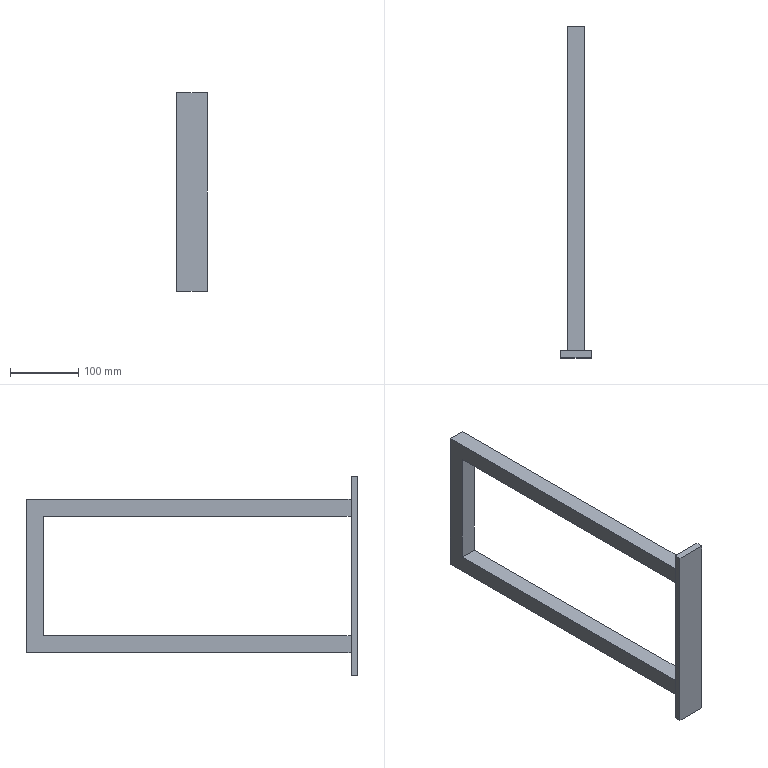Part | SolidWorks | features BaseBody 1 | 1 solid | 14 faces | box 45 x 485 x 290 mm | volume 833625 mm3 | plane 14
STEP:
#1=CARTESIAN_POINT('',(12.5,485.,-112.5));
#2=VERTEX_POINT('',#1);
#3=CARTESIAN_POINT('',(12.5,10.,-112.5));
#4=VERTEX_POINT('',#3);
#5=CARTESIAN_POINT('',(12.5,460.,-112.5));
#6=DIRECTION('',(0.,-1.,0.));
#7=VECTOR('',#6,1000.);
#8=LINE('',#5,#7);
#9=EDGE_CURVE('',#2,#4,#8,.T.);
#10=ORIENTED_EDGE('',*,*,#9,.F.);
#11=CARTESIAN_POINT('',(12.5,485.,112.5));
#12=VERTEX_POINT('',#11);
#13=CARTESIAN_POINT('',(12.5,485.,-112.5));
#14=DIRECTION('',(0.,0.,-1.));
#15=VECTOR('',#14,1000.);
#16=LINE('',#13,#15);
#17=EDGE_CURVE('',#12,#2,#16,.T.);
#18=ORIENTED_EDGE('',*,*,#17,.F.);
#19=CARTESIAN_POINT('',(12.5,10.,112.5));
#20=VERTEX_POINT('',#19);
#21=CARTESIAN_POINT('',(12.5,460.,112.5));
#22=DIRECTION('',(0.,1.,0.));
#23=VECTOR('',#22,1000.);
#24=LINE('',#21,#23);
#25=EDGE_CURVE('',#20,#12,#24,.T.);
#26=ORIENTED_EDGE('',*,*,#25,.F.);
#27=CARTESIAN_POINT('',(12.5,10.,87.5));
#28=VERTEX_POINT('',#27);
#29=CARTESIAN_POINT('',(12.5,10.,-112.5));
#30=DIRECTION('',(0.,0.,1.));
#31=VECTOR('',#30,1000.);
#32=LINE('',#29,#31);
#33=EDGE_CURVE('',#28,#20,#32,.T.);
#34=ORIENTED_EDGE('',*,*,#33,.F.);
#35=CARTESIAN_POINT('',(12.5,460.,87.5));
#36=VERTEX_POINT('',#35);
#37=CARTESIAN_POINT('',(12.5,460.,87.5));
#38=DIRECTION('',(0.,-1.,0.));
#39=VECTOR('',#38,1000.);
#40=LINE('',#37,#39);
#41=EDGE_CURVE('',#36,#28,#40,.T.);
#42=ORIENTED_EDGE('',*,*,#41,.F.);
#43=CARTESIAN_POINT('',(12.5,460.,-87.5));
#44=VERTEX_POINT('',#43);
#45=CARTESIAN_POINT('',(12.5,460.,-112.5));
#46=DIRECTION('',(0.,0.,1.));
#47=VECTOR('',#46,1000.);
#48=LINE('',#45,#47);
#49=EDGE_CURVE('',#44,#36,#48,.T.);
#50=ORIENTED_EDGE('',*,*,#49,.F.);
#51=CARTESIAN_POINT('',(12.5,10.,-87.5));
#52=VERTEX_POINT('',#51);
#53=CARTESIAN_POINT('',(12.5,460.,-87.5));
#54=DIRECTION('',(0.,1.,0.));
#55=VECTOR('',#54,1000.);
#56=LINE('',#53,#55);
#57=EDGE_CURVE('',#52,#44,#56,.T.);
#58=ORIENTED_EDGE('',*,*,#57,.F.);
#59=CARTESIAN_POINT('',(12.5,10.,-112.5));
#60=DIRECTION('',(0.,0.,1.));
#61=VECTOR('',#60,1000.);
#62=LINE('',#59,#61);
#63=EDGE_CURVE('',#4,#52,#62,.T.);
#64=ORIENTED_EDGE('',*,*,#63,.F.);
#65=EDGE_LOOP('',(#10,#18,#26,#34,#42,#50,#58,#64));
#66=FACE_OUTER_BOUND('',#65,.T.);
#67=CARTESIAN_POINT('',(12.5,460.,-112.5));
#68=DIRECTION('',(-1.,0.,0.));
#69=DIRECTION('',(0.,0.,1.));
#70=AXIS2_PLACEMENT_3D('',#67,#68,#69);
#71=PLANE('',#70);
#72=ADVANCED_FACE('',(#66),#71,.F.);
#73=CARTESIAN_POINT('',(-12.5,10.,112.5));
#74=VERTEX_POINT('',#73);
#75=CARTESIAN_POINT('',(0.,10.,112.5));
#76=DIRECTION('',(-1.,0.,0.));
#77=VECTOR('',#76,1000.);
#78=LINE('',#75,#77);
#79=EDGE_CURVE('',#20,#74,#78,.T.);
#80=ORIENTED_EDGE('',*,*,#79,.T.);
#81=CARTESIAN_POINT('',(-12.5,10.,87.5));
#82=VERTEX_POINT('',#81);
#83=CARTESIAN_POINT('',(-12.5,10.,0.));
#84=DIRECTION('',(0.,0.,-1.));
#85=VECTOR('',#84,1000.);
#86=LINE('',#83,#85);
#87=EDGE_CURVE('',#74,#82,#86,.T.);
#88=ORIENTED_EDGE('',*,*,#87,.T.);
#89=CARTESIAN_POINT('',(0.,10.,87.5));
#90=DIRECTION('',(1.,0.,0.));
#91=VECTOR('',#90,1000.);
#92=LINE('',#89,#91);
#93=EDGE_CURVE('',#82,#28,#92,.T.);
#94=ORIENTED_EDGE('',*,*,#93,.T.);
#95=ORIENTED_EDGE('',*,*,#33,.T.);
#96=EDGE_LOOP('',(#80,#88,#94,#95));
#97=FACE_BOUND('',#96,.T.);
#98=CARTESIAN_POINT('',(-12.5,10.,-87.5));
#99=VERTEX_POINT('',#98);
#100=CARTESIAN_POINT('',(0.,10.,-87.5));
#101=DIRECTION('',(-1.,0.,0.));
#102=VECTOR('',#101,1000.);
#103=LINE('',#100,#102);
#104=EDGE_CURVE('',#52,#99,#103,.T.);
#105=ORIENTED_EDGE('',*,*,#104,.T.);
#106=CARTESIAN_POINT('',(-12.5,10.,-112.5));
#107=VERTEX_POINT('',#106);
#108=CARTESIAN_POINT('',(-12.5,10.,0.));
#109=DIRECTION('',(0.,0.,-1.));
#110=VECTOR('',#109,1000.);
#111=LINE('',#108,#110);
#112=EDGE_CURVE('',#99,#107,#111,.T.);
#113=ORIENTED_EDGE('',*,*,#112,.T.);
#114=CARTESIAN_POINT('',(0.,10.,-112.5));
#115=DIRECTION('',(1.,0.,0.));
#116=VECTOR('',#115,1000.);
#117=LINE('',#114,#116);
#118=EDGE_CURVE('',#107,#4,#117,.T.);
#119=ORIENTED_EDGE('',*,*,#118,.T.);
#120=ORIENTED_EDGE('',*,*,#63,.T.);
#121=EDGE_LOOP('',(#105,#113,#119,#120));
#122=FACE_BOUND('',#121,.T.);
#123=CARTESIAN_POINT('',(22.5,10.,145.));
#124=VERTEX_POINT('',#123);
#125=CARTESIAN_POINT('',(22.5,10.,-145.));
#126=VERTEX_POINT('',#125);
#127=CARTESIAN_POINT('',(22.5,10.,0.));
#128=DIRECTION('',(0.,0.,-1.));
#129=VECTOR('',#128,1000.);
#130=LINE('',#127,#129);
#131=EDGE_CURVE('',#124,#126,#130,.T.);
#132=ORIENTED_EDGE('',*,*,#131,.T.);
#133=CARTESIAN_POINT('',(-22.5,10.,-145.));
#134=VERTEX_POINT('',#133);
#135=CARTESIAN_POINT('',(0.,10.,-145.));
#136=DIRECTION('',(-1.,0.,0.));
#137=VECTOR('',#136,1000.);
#138=LINE('',#135,#137);
#139=EDGE_CURVE('',#126,#134,#138,.T.);
#140=ORIENTED_EDGE('',*,*,#139,.T.);
#141=CARTESIAN_POINT('',(-22.5,10.,145.));
#142=VERTEX_POINT('',#141);
#143=CARTESIAN_POINT('',(-22.5,10.,0.));
#144=DIRECTION('',(0.,0.,1.));
#145=VECTOR('',#144,1000.);
#146=LINE('',#143,#145);
#147=EDGE_CURVE('',#134,#142,#146,.T.);
#148=ORIENTED_EDGE('',*,*,#147,.T.);
#149=CARTESIAN_POINT('',(0.,10.,145.));
#150=DIRECTION('',(1.,0.,0.));
#151=VECTOR('',#150,1000.);
#152=LINE('',#149,#151);
#153=EDGE_CURVE('',#142,#124,#152,.T.);
#154=ORIENTED_EDGE('',*,*,#153,.T.);
#155=EDGE_LOOP('',(#132,#140,#148,#154));
#156=FACE_OUTER_BOUND('',#155,.T.);
#157=CARTESIAN_POINT('',(0.,10.,0.));
#158=DIRECTION('',(0.,1.,0.));
#159=DIRECTION('',(0.,0.,1.));
#160=AXIS2_PLACEMENT_3D('',#157,#158,#159);
#161=PLANE('',#160);
#162=ADVANCED_FACE('',(#97,#122,#156),#161,.T.);
#163=CARTESIAN_POINT('',(-12.5,485.,-112.5));
#164=VERTEX_POINT('',#163);
#165=CARTESIAN_POINT('',(-12.5,460.,-112.5));
#166=DIRECTION('',(0.,-1.,0.));
#167=VECTOR('',#166,1000.);
#168=LINE('',#165,#167);
#169=EDGE_CURVE('',#164,#107,#168,.T.);
#170=ORIENTED_EDGE('',*,*,#169,.F.);
#171=CARTESIAN_POINT('',(-12.5,485.,-112.5));
#172=DIRECTION('',(-1.,0.,0.));
#173=VECTOR('',#172,1000.);
#174=LINE('',#171,#173);
#175=EDGE_CURVE('',#2,#164,#174,.T.);
#176=ORIENTED_EDGE('',*,*,#175,.F.);
#177=ORIENTED_EDGE('',*,*,#9,.T.);
#178=ORIENTED_EDGE('',*,*,#118,.F.);
#179=EDGE_LOOP('',(#170,#176,#177,#178));
#180=FACE_OUTER_BOUND('',#179,.T.);
#181=CARTESIAN_POINT('',(-12.5,460.,-112.5));
#182=DIRECTION('',(0.,0.,1.));
#183=DIRECTION('',(1.,0.,0.));
#184=AXIS2_PLACEMENT_3D('',#181,#182,#183);
#185=PLANE('',#184);
#186=ADVANCED_FACE('',(#180),#185,.F.);
#187=ORIENTED_EDGE('',*,*,#175,.T.);
#188=CARTESIAN_POINT('',(-12.5,485.,112.5));
#189=VERTEX_POINT('',#188);
#190=CARTESIAN_POINT('',(-12.5,485.,-112.5));
#191=DIRECTION('',(0.,0.,1.));
#192=VECTOR('',#191,1000.);
#193=LINE('',#190,#192);
#194=EDGE_CURVE('',#164,#189,#193,.T.);
#195=ORIENTED_EDGE('',*,*,#194,.T.);
#196=CARTESIAN_POINT('',(-12.5,485.,112.5));
#197=DIRECTION('',(1.,0.,0.));
#198=VECTOR('',#197,1000.);
#199=LINE('',#196,#198);
#200=EDGE_CURVE('',#189,#12,#199,.T.);
#201=ORIENTED_EDGE('',*,*,#200,.T.);
#202=ORIENTED_EDGE('',*,*,#17,.T.);
#203=EDGE_LOOP('',(#187,#195,#201,#202));
#204=FACE_OUTER_BOUND('',#203,.T.);
#205=CARTESIAN_POINT('',(-12.5,485.,-112.5));
#206=DIRECTION('',(0.,1.,0.));
#207=DIRECTION('',(0.,0.,1.));
#208=AXIS2_PLACEMENT_3D('',#205,#206,#207);
#209=PLANE('',#208);
#210=ADVANCED_FACE('',(#204),#209,.T.);
#211=ORIENTED_EDGE('',*,*,#25,.T.);
#212=ORIENTED_EDGE('',*,*,#200,.F.);
#213=CARTESIAN_POINT('',(-12.5,460.,112.5));
#214=DIRECTION('',(0.,1.,0.));
#215=VECTOR('',#214,1000.);
#216=LINE('',#213,#215);
#217=EDGE_CURVE('',#74,#189,#216,.T.);
#218=ORIENTED_EDGE('',*,*,#217,.F.);
#219=ORIENTED_EDGE('',*,*,#79,.F.);
#220=EDGE_LOOP('',(#211,#212,#218,#219));
#221=FACE_OUTER_BOUND('',#220,.T.);
#222=CARTESIAN_POINT('',(-12.5,460.,112.5));
#223=DIRECTION('',(0.,0.,-1.));
#224=DIRECTION('',(-1.,0.,0.));
#225=AXIS2_PLACEMENT_3D('',#222,#223,#224);
#226=PLANE('',#225);
#227=ADVANCED_FACE('',(#221),#226,.F.);
#228=CARTESIAN_POINT('',(-12.5,460.,87.5));
#229=VERTEX_POINT('',#228);
#230=CARTESIAN_POINT('',(-12.5,460.,87.5));
#231=DIRECTION('',(0.,-1.,0.));
#232=VECTOR('',#231,1000.);
#233=LINE('',#230,#232);
#234=EDGE_CURVE('',#229,#82,#233,.T.);
#235=ORIENTED_EDGE('',*,*,#234,.F.);
#236=CARTESIAN_POINT('',(-12.5,460.,87.5));
#237=DIRECTION('',(-1.,0.,0.));
#238=VECTOR('',#237,1000.);
#239=LINE('',#236,#238);
#240=EDGE_CURVE('',#36,#229,#239,.T.);
#241=ORIENTED_EDGE('',*,*,#240,.F.);
#242=ORIENTED_EDGE('',*,*,#41,.T.);
#243=ORIENTED_EDGE('',*,*,#93,.F.);
#244=EDGE_LOOP('',(#235,#241,#242,#243));
#245=FACE_OUTER_BOUND('',#244,.T.);
#246=CARTESIAN_POINT('',(-12.5,460.,87.5));
#247=DIRECTION('',(0.,0.,1.));
#248=DIRECTION('',(1.,0.,0.));
#249=AXIS2_PLACEMENT_3D('',#246,#247,#248);
#250=PLANE('',#249);
#251=ADVANCED_FACE('',(#245),#250,.F.);
#252=ORIENTED_EDGE('',*,*,#49,.T.);
#253=ORIENTED_EDGE('',*,*,#240,.T.);
#254=CARTESIAN_POINT('',(-12.5,460.,-87.5));
#255=VERTEX_POINT('',#254);
#256=CARTESIAN_POINT('',(-12.5,460.,-112.5));
#257=DIRECTION('',(0.,0.,-1.));
#258=VECTOR('',#257,1000.);
#259=LINE('',#256,#258);
#260=EDGE_CURVE('',#229,#255,#259,.T.);
#261=ORIENTED_EDGE('',*,*,#260,.T.);
#262=CARTESIAN_POINT('',(-12.5,460.,-87.5));
#263=DIRECTION('',(1.,0.,0.));
#264=VECTOR('',#263,1000.);
#265=LINE('',#262,#264);
#266=EDGE_CURVE('',#255,#44,#265,.T.);
#267=ORIENTED_EDGE('',*,*,#266,.T.);
#268=EDGE_LOOP('',(#252,#253,#261,#267));
#269=FACE_OUTER_BOUND('',#268,.T.);
#270=CARTESIAN_POINT('',(-12.5,460.,-112.5));
#271=DIRECTION('',(0.,-1.,0.));
#272=DIRECTION('',(0.,0.,-1.));
#273=AXIS2_PLACEMENT_3D('',#270,#271,#272);
#274=PLANE('',#273);
#275=ADVANCED_FACE('',(#269),#274,.T.);
#276=ORIENTED_EDGE('',*,*,#57,.T.);
#277=ORIENTED_EDGE('',*,*,#266,.F.);
#278=CARTESIAN_POINT('',(-12.5,460.,-87.5));
#279=DIRECTION('',(0.,1.,0.));
#280=VECTOR('',#279,1000.);
#281=LINE('',#278,#280);
#282=EDGE_CURVE('',#99,#255,#281,.T.);
#283=ORIENTED_EDGE('',*,*,#282,.F.);
#284=ORIENTED_EDGE('',*,*,#104,.F.);
#285=EDGE_LOOP('',(#276,#277,#283,#284));
#286=FACE_OUTER_BOUND('',#285,.T.);
#287=CARTESIAN_POINT('',(-12.5,460.,-87.5));
#288=DIRECTION('',(0.,0.,-1.));
#289=DIRECTION('',(-1.,0.,0.));
#290=AXIS2_PLACEMENT_3D('',#287,#288,#289);
#291=PLANE('',#290);
#292=ADVANCED_FACE('',(#286),#291,.F.);
#293=ORIENTED_EDGE('',*,*,#282,.T.);
#294=ORIENTED_EDGE('',*,*,#260,.F.);
#295=ORIENTED_EDGE('',*,*,#234,.T.);
#296=ORIENTED_EDGE('',*,*,#87,.F.);
#297=ORIENTED_EDGE('',*,*,#217,.T.);
#298=ORIENTED_EDGE('',*,*,#194,.F.);
#299=ORIENTED_EDGE('',*,*,#169,.T.);
#300=ORIENTED_EDGE('',*,*,#112,.F.);
#301=EDGE_LOOP('',(#293,#294,#295,#296,#297,#298,#299,#300));
#302=FACE_OUTER_BOUND('',#301,.T.);
#303=CARTESIAN_POINT('',(-12.5,460.,-112.5));
#304=DIRECTION('',(1.,0.,0.));
#305=DIRECTION('',(0.,0.,-1.));
#306=AXIS2_PLACEMENT_3D('',#303,#304,#305);
#307=PLANE('',#306);
#308=ADVANCED_FACE('',(#302),#307,.F.);
#309=CARTESIAN_POINT('',(-22.5,0.,-145.));
#310=VERTEX_POINT('',#309);
#311=CARTESIAN_POINT('',(-22.5,10.,-145.));
#312=DIRECTION('',(0.,-1.,0.));
#313=VECTOR('',#312,1000.);
#314=LINE('',#311,#313);
#315=EDGE_CURVE('',#134,#310,#314,.T.);
#316=ORIENTED_EDGE('',*,*,#315,.F.);
#317=ORIENTED_EDGE('',*,*,#139,.F.);
#318=CARTESIAN_POINT('',(22.5,0.,-145.));
#319=VERTEX_POINT('',#318);
#320=CARTESIAN_POINT('',(22.5,10.,-145.));
#321=DIRECTION('',(0.,1.,0.));
#322=VECTOR('',#321,1000.);
#323=LINE('',#320,#322);
#324=EDGE_CURVE('',#319,#126,#323,.T.);
#325=ORIENTED_EDGE('',*,*,#324,.F.);
#326=CARTESIAN_POINT('',(22.5,0.,-145.));
#327=DIRECTION('',(1.,0.,0.));
#328=VECTOR('',#327,1000.);
#329=LINE('',#326,#328);
#330=EDGE_CURVE('',#310,#319,#329,.T.);
#331=ORIENTED_EDGE('',*,*,#330,.F.);
#332=EDGE_LOOP('',(#316,#317,#325,#331));
#333=FACE_OUTER_BOUND('',#332,.T.);
#334=CARTESIAN_POINT('',(22.5,10.,-145.));
#335=DIRECTION('',(0.,0.,1.));
#336=DIRECTION('',(1.,0.,0.));
#337=AXIS2_PLACEMENT_3D('',#334,#335,#336);
#338=PLANE('',#337);
#339=ADVANCED_FACE('',(#333),#338,.F.);
#340=ORIENTED_EDGE('',*,*,#324,.T.);
#341=ORIENTED_EDGE('',*,*,#131,.F.);
#342=CARTESIAN_POINT('',(22.5,0.,145.));
#343=VERTEX_POINT('',#342);
#344=CARTESIAN_POINT('',(22.5,10.,145.));
#345=DIRECTION('',(0.,1.,0.));
#346=VECTOR('',#345,1000.);
#347=LINE('',#344,#346);
#348=EDGE_CURVE('',#343,#124,#347,.T.);
#349=ORIENTED_EDGE('',*,*,#348,.F.);
#350=CARTESIAN_POINT('',(22.5,0.,145.));
#351=DIRECTION('',(0.,0.,1.));
#352=VECTOR('',#351,1000.);
#353=LINE('',#350,#352);
#354=EDGE_CURVE('',#319,#343,#353,.T.);
#355=ORIENTED_EDGE('',*,*,#354,.F.);
#356=EDGE_LOOP('',(#340,#341,#349,#355));
#357=FACE_OUTER_BOUND('',#356,.T.);
#358=CARTESIAN_POINT('',(22.5,10.,145.));
#359=DIRECTION('',(-1.,0.,0.));
#360=DIRECTION('',(0.,0.,1.));
#361=AXIS2_PLACEMENT_3D('',#358,#359,#360);
#362=PLANE('',#361);
#363=ADVANCED_FACE('',(#357),#362,.F.);
#364=ORIENTED_EDGE('',*,*,#348,.T.);
#365=ORIENTED_EDGE('',*,*,#153,.F.);
#366=CARTESIAN_POINT('',(-22.5,0.,145.));
#367=VERTEX_POINT('',#366);
#368=CARTESIAN_POINT('',(-22.5,10.,145.));
#369=DIRECTION('',(0.,1.,0.));
#370=VECTOR('',#369,1000.);
#371=LINE('',#368,#370);
#372=EDGE_CURVE('',#367,#142,#371,.T.);
#373=ORIENTED_EDGE('',*,*,#372,.F.);
#374=CARTESIAN_POINT('',(22.5,0.,145.));
#375=DIRECTION('',(-1.,0.,0.));
#376=VECTOR('',#375,1000.);
#377=LINE('',#374,#376);
#378=EDGE_CURVE('',#343,#367,#377,.T.);
#379=ORIENTED_EDGE('',*,*,#378,.F.);
#380=EDGE_LOOP('',(#364,#365,#373,#379));
#381=FACE_OUTER_BOUND('',#380,.T.);
#382=CARTESIAN_POINT('',(22.5,10.,145.));
#383=DIRECTION('',(0.,0.,-1.));
#384=DIRECTION('',(-1.,0.,0.));
#385=AXIS2_PLACEMENT_3D('',#382,#383,#384);
#386=PLANE('',#385);
#387=ADVANCED_FACE('',(#381),#386,.F.);
#388=ORIENTED_EDGE('',*,*,#372,.T.);
#389=ORIENTED_EDGE('',*,*,#147,.F.);
#390=ORIENTED_EDGE('',*,*,#315,.T.);
#391=CARTESIAN_POINT('',(-22.5,0.,145.));
#392=DIRECTION('',(0.,0.,-1.));
#393=VECTOR('',#392,1000.);
#394=LINE('',#391,#393);
#395=EDGE_CURVE('',#367,#310,#394,.T.);
#396=ORIENTED_EDGE('',*,*,#395,.F.);
#397=EDGE_LOOP('',(#388,#389,#390,#396));
#398=FACE_OUTER_BOUND('',#397,.T.);
#399=CARTESIAN_POINT('',(-22.5,10.,145.));
#400=DIRECTION('',(1.,0.,0.));
#401=DIRECTION('',(0.,0.,-1.));
#402=AXIS2_PLACEMENT_3D('',#399,#400,#401);
#403=PLANE('',#402);
#404=ADVANCED_FACE('',(#398),#403,.F.);
#405=ORIENTED_EDGE('',*,*,#330,.T.);
#406=ORIENTED_EDGE('',*,*,#354,.T.);
#407=ORIENTED_EDGE('',*,*,#378,.T.);
#408=ORIENTED_EDGE('',*,*,#395,.T.);
#409=EDGE_LOOP('',(#405,#406,#407,#408));
#410=FACE_OUTER_BOUND('',#409,.T.);
#411=CARTESIAN_POINT('',(0.,0.,0.));
#412=DIRECTION('',(0.,1.,0.));
#413=DIRECTION('',(0.,0.,1.));
#414=AXIS2_PLACEMENT_3D('',#411,#412,#413);
#415=PLANE('',#414);
#416=ADVANCED_FACE('',(#410),#415,.F.);
#417=CLOSED_SHELL('',(#72,#162,#186,#210,#227,#251,#275,#292,#308,#339,#363,#387,#404,#416));
#418=MANIFOLD_SOLID_BREP('',#417);
#419=CARTESIAN_POINT('',(0.,0.,0.));
#420=DIRECTION('',(0.,0.,1.));
#421=DIRECTION('',(1.,0.,0.));
#422=AXIS2_PLACEMENT_3D('',#419,#420,#421);
#423=(LENGTH_UNIT()NAMED_UNIT(*)SI_UNIT(.MILLI.,.METRE.));
#424=UNCERTAINTY_MEASURE_WITH_UNIT(LENGTH_MEASURE(0.00001),#423,'','');
#425=(NAMED_UNIT(*)PLANE_ANGLE_UNIT()SI_UNIT($,.RADIAN.));
#426=(NAMED_UNIT(*)SI_UNIT($,.STERADIAN.)SOLID_ANGLE_UNIT());
#427=(GEOMETRIC_REPRESENTATION_CONTEXT(3)GLOBAL_UNCERTAINTY_ASSIGNED_CONTEXT((#424))GLOBAL_UNIT_ASSIGNED_CONTEXT((#423,#425,#426))REPRESENTATION_CONTEXT('',''));
#428=ADVANCED_BREP_SHAPE_REPRESENTATION('',(#418,#422),#427);